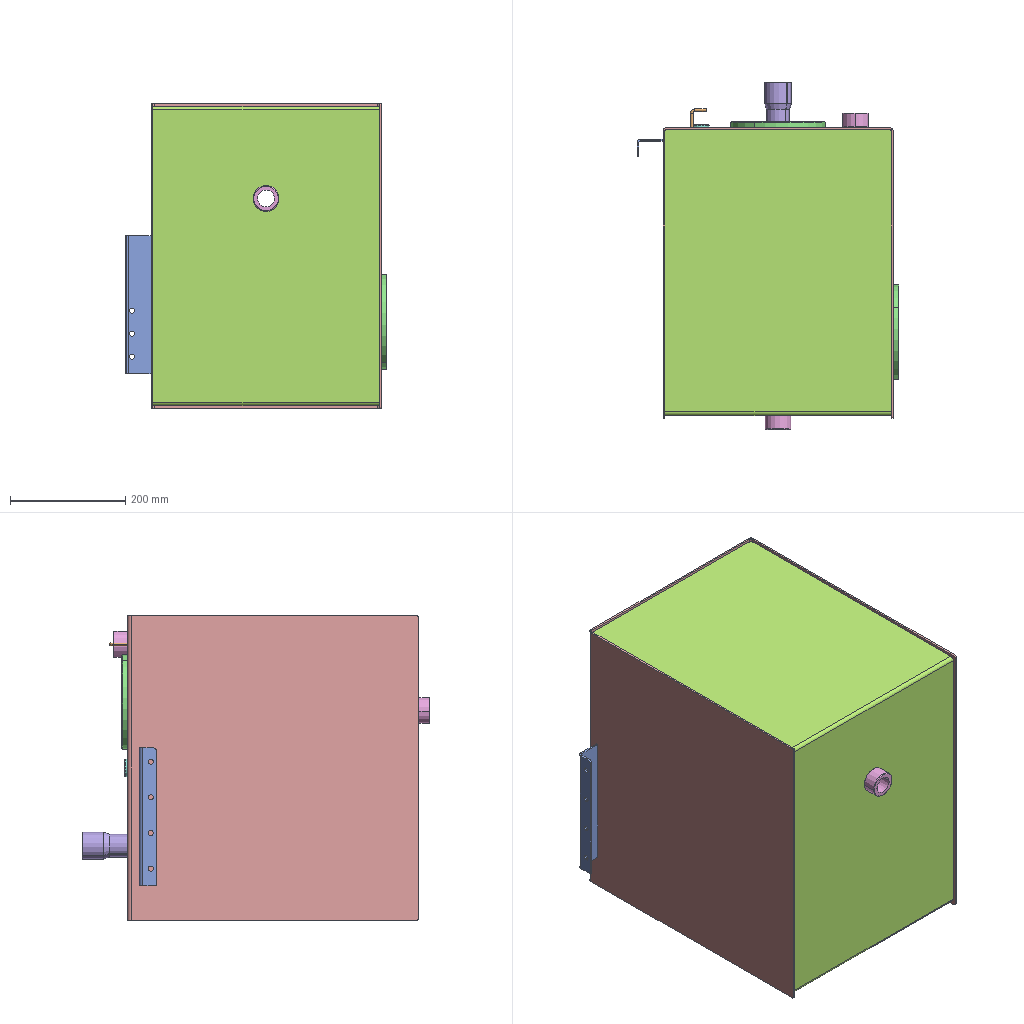Assembly | SolidWorks | 8 different items | 10 placed | box 455 x 604 x 530 mm
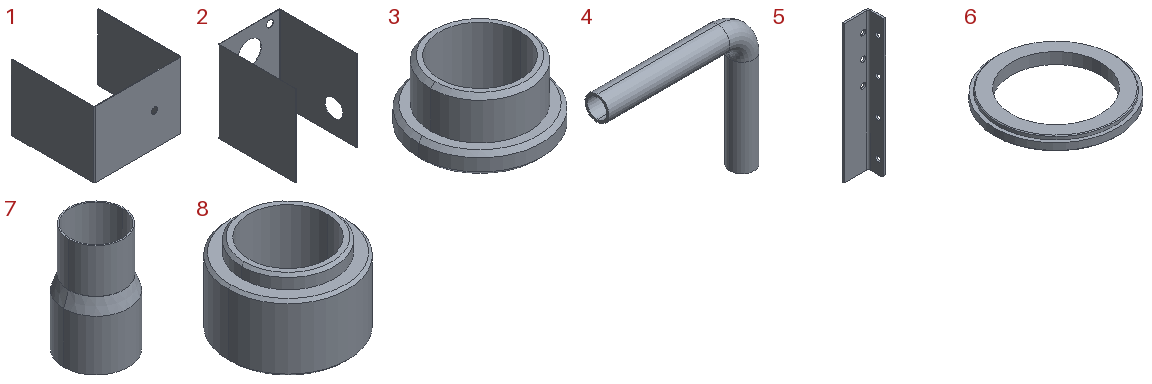Parts list (item | quantity | size | volume | features):
1 | x1 | 520 x 497 x 394 mm | 1774939 mm3 | features ICE 2, FlatPattern 1, SMBaseFlange 1, SheetMetal 1
2 | x1 | 400 x 505 x 530 mm | 2126539 mm3 | features ICE 4, Cut 2, FlatPattern 1, SMBaseFlange 1, SheetMetal 1
3 | x1 | 30 x 30 x 15 mm | 3311 mm3 | features Chamfer 1, Extrusion 1, ICE 1
4 | x1 | 32.5 x 5 x 27.5 mm | 373.603 mm3 | features Sweep 1
5 | x1 | 45 x 30 x 240 mm | 49097 mm3 | features ICE 2, Fillet 1, FlatPattern 1, SMBaseFlange 1, SheetMetal 1
6 | x2 | 165 x 165 x 15 mm | 136481 mm3 | features 3DProfileFeature 1, Chamfer 1, Extrusion 1, HoleWzd 1, ICE 1
7 | x1 | 47 x 47 x 79 mm | 10172 mm3 | features 3DProfileFeature 2, ICE 2, NetBlend 1, NetBlendCut 1
8 | x2 | 45 x 45 x 30 mm | 23873 mm3 | features Chamfer 1, Extrusion 1, ICE 1
Mates (type | each side: item.copy, entity, surface, feature):
Coincident | 2.1 face plane Base-Flange1 | 1.1 face plane Base-Flange1 | 2 times
DistanceDim | 1.1 face plane Base-Flange1 | 2.1 face plane Base-Flange1
Coincident | 2.1 face plane Base-Flange1 | 5.1 face plane Base-Flange1
DistanceDim | 5.1 face plane Base-Flange1 | 2.1 face plane Base-Flange1 | 2 times
Concentric | 1.1 edge | 8.1 edge
Coincident | 1.1 face plane Base-Flange1 | 8.1 face plane Boss-Extrude1
Concentric | 2.1 edge | 8.2 edge
Coincident | 2.1 face plane Base-Flange1 | 8.2 face plane Boss-Extrude1
Concentric | 2.1 edge | 3.1 edge
Coincident | 2.1 face plane Base-Flange1 | 3.1 face plane Boss-Extrude1
Concentric | 2.1 edge | 4.1 edge
Coincident | 2.1 face plane Base-Flange1 | 4.1 face plane Sweep1
Parallel | 2.1 face plane Base-Flange1 | 4.1 face plane Sweep1
Concentric | 2.1 edge | 7.1 edge
Coincident | 2.1 face plane Base-Flange1 | 7.1 face plane Boss-Extrude2
Coincident | 2.1 face plane Base-Flange1 | 6.1 face plane Boss-Extrude1
Concentric | 2.1 edge | 6.1 edge
Coincident | 2.1 face plane Base-Flange1 | 6.2 face plane Boss-Extrude1
Concentric | 2.1 edge | 6.2 edge